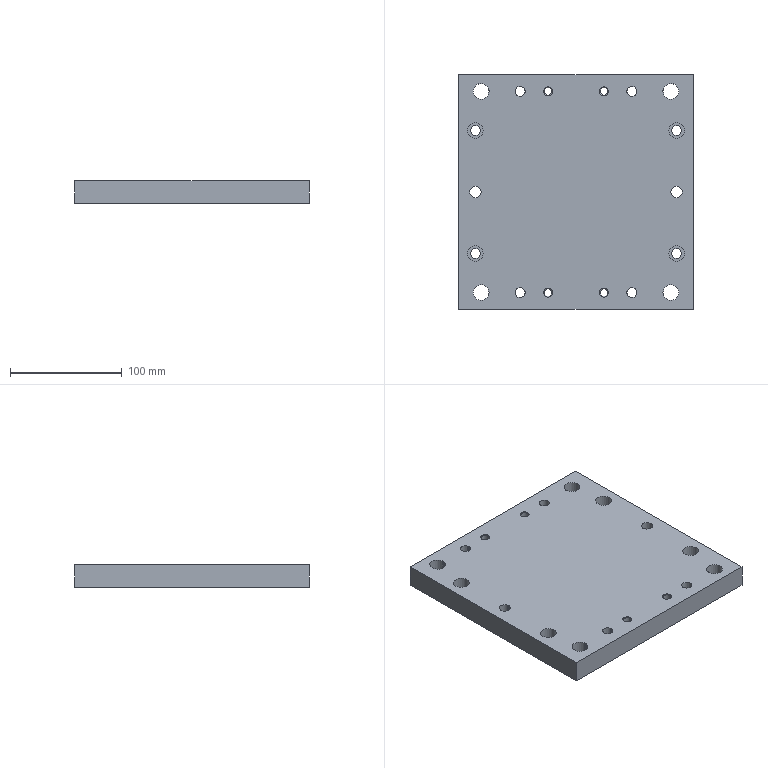Part | STEP file | YBQDJ-YL-1 | 1 solid | 78 faces | box 210 x 210 x 20 mm | volume 848713 mm3 | cylinder 52 | cone 16 | plane 10 | commonest cylinder face diameters 4 x20 1 x10 14 x8 6.8 x4 8.7 x4 9 x4